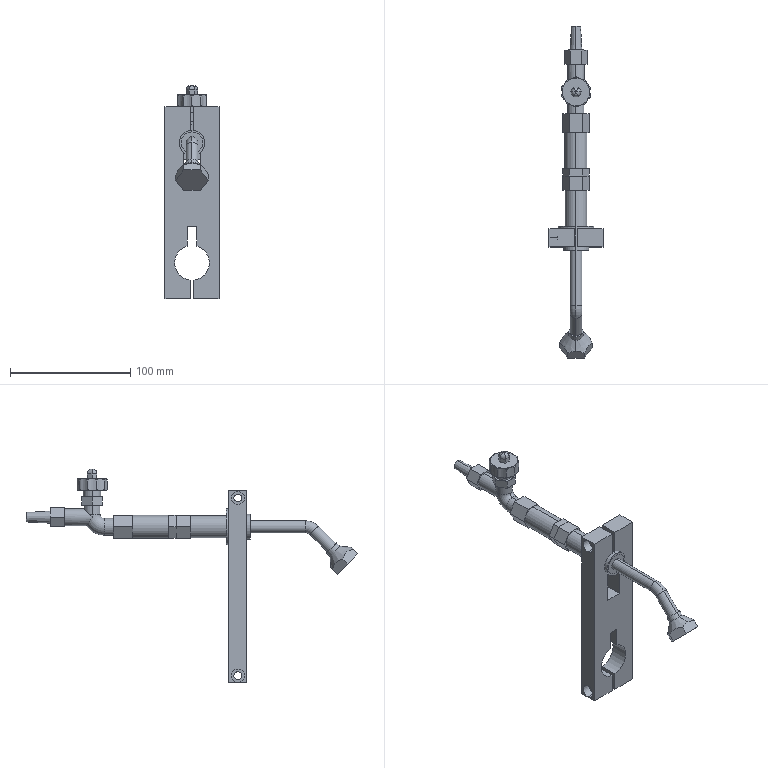Part | STEP file | DH24-32 | 8 solids | 169 faces | box 45 x 276.598 x 178 mm | volume 145916 mm3 | plane 85 | cylinder 40 | torus 24 | spline 16 | cone 4 | commonest cylinder face diameters 6.6 x8 14 x6 10 x4 11 x4 18 x4 21 x4